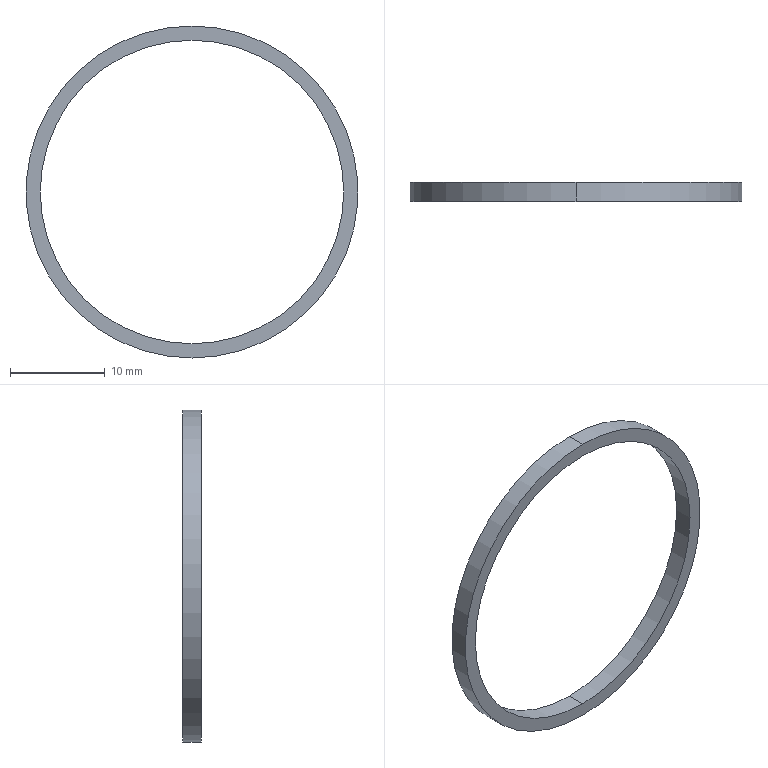Part | SolidWorks | features Extrusion 1 | 1 solid | 6 faces | box 35 x 2 x 35 mm | volume 315.73 mm3 | cylinder 4 | plane 2 | commonest cylinder face diameters 32 x2 35 x2
STEP:
#1=CARTESIAN_POINT('',(0.,1.,-16.));
#2=VERTEX_POINT('',#1);
#3=CARTESIAN_POINT('',(0.,1.,16.));
#4=VERTEX_POINT('',#3);
#5=CARTESIAN_POINT('',(0.,1.,0.));
#6=DIRECTION('',(0.,1.,0.));
#7=DIRECTION('',(0.,0.,1.));
#8=AXIS2_PLACEMENT_3D('',#5,#6,#7);
#9=CIRCLE('',#8,16.);
#10=EDGE_CURVE('',#2,#4,#9,.T.);
#11=ORIENTED_EDGE('',*,*,#10,.T.);
#12=CARTESIAN_POINT('',(0.,-1.,16.));
#13=VERTEX_POINT('',#12);
#14=CARTESIAN_POINT('',(0.,1.,16.));
#15=DIRECTION('',(0.,-1.,0.));
#16=VECTOR('',#15,1000.);
#17=LINE('',#14,#16);
#18=EDGE_CURVE('',#4,#13,#17,.T.);
#19=ORIENTED_EDGE('',*,*,#18,.T.);
#20=CARTESIAN_POINT('',(0.,-1.,-16.));
#21=VERTEX_POINT('',#20);
#22=CARTESIAN_POINT('',(0.,-1.,0.));
#23=DIRECTION('',(0.,1.,0.));
#24=DIRECTION('',(0.,0.,1.));
#25=AXIS2_PLACEMENT_3D('',#22,#23,#24);
#26=CIRCLE('',#25,16.);
#27=EDGE_CURVE('',#21,#13,#26,.T.);
#28=ORIENTED_EDGE('',*,*,#27,.F.);
#29=CARTESIAN_POINT('',(0.,1.,-16.));
#30=DIRECTION('',(0.,-1.,0.));
#31=VECTOR('',#30,1000.);
#32=LINE('',#29,#31);
#33=EDGE_CURVE('',#2,#21,#32,.T.);
#34=ORIENTED_EDGE('',*,*,#33,.F.);
#35=EDGE_LOOP('',(#11,#19,#28,#34));
#36=FACE_OUTER_BOUND('',#35,.T.);
#37=CARTESIAN_POINT('',(0.,1.,0.));
#38=DIRECTION('',(0.,-1.,0.));
#39=DIRECTION('',(0.,0.,-1.));
#40=AXIS2_PLACEMENT_3D('',#37,#38,#39);
#41=CYLINDRICAL_SURFACE('',#40,16.);
#42=ADVANCED_FACE('',(#36),#41,.F.);
#43=CARTESIAN_POINT('',(0.,1.,17.5));
#44=VERTEX_POINT('',#43);
#45=CARTESIAN_POINT('',(0.,1.,-17.5));
#46=VERTEX_POINT('',#45);
#47=CARTESIAN_POINT('',(0.,1.,0.));
#48=DIRECTION('',(0.,1.,0.));
#49=DIRECTION('',(0.,0.,1.));
#50=AXIS2_PLACEMENT_3D('',#47,#48,#49);
#51=CIRCLE('',#50,17.5);
#52=EDGE_CURVE('',#44,#46,#51,.T.);
#53=ORIENTED_EDGE('',*,*,#52,.F.);
#54=CARTESIAN_POINT('',(0.,-1.,17.5));
#55=VERTEX_POINT('',#54);
#56=CARTESIAN_POINT('',(0.,1.,17.5));
#57=DIRECTION('',(0.,-1.,0.));
#58=VECTOR('',#57,1000.);
#59=LINE('',#56,#58);
#60=EDGE_CURVE('',#44,#55,#59,.T.);
#61=ORIENTED_EDGE('',*,*,#60,.T.);
#62=CARTESIAN_POINT('',(0.,-1.,-17.5));
#63=VERTEX_POINT('',#62);
#64=CARTESIAN_POINT('',(0.,-1.,0.));
#65=DIRECTION('',(0.,1.,0.));
#66=DIRECTION('',(0.,0.,1.));
#67=AXIS2_PLACEMENT_3D('',#64,#65,#66);
#68=CIRCLE('',#67,17.5);
#69=EDGE_CURVE('',#55,#63,#68,.T.);
#70=ORIENTED_EDGE('',*,*,#69,.T.);
#71=CARTESIAN_POINT('',(0.,1.,-17.5));
#72=DIRECTION('',(0.,-1.,0.));
#73=VECTOR('',#72,1000.);
#74=LINE('',#71,#73);
#75=EDGE_CURVE('',#46,#63,#74,.T.);
#76=ORIENTED_EDGE('',*,*,#75,.F.);
#77=EDGE_LOOP('',(#53,#61,#70,#76));
#78=FACE_OUTER_BOUND('',#77,.T.);
#79=CARTESIAN_POINT('',(0.,1.,0.));
#80=DIRECTION('',(0.,-1.,0.));
#81=DIRECTION('',(0.,0.,-1.));
#82=AXIS2_PLACEMENT_3D('',#79,#80,#81);
#83=CYLINDRICAL_SURFACE('',#82,17.5);
#84=ADVANCED_FACE('',(#78),#83,.T.);
#85=CARTESIAN_POINT('',(0.,1.,0.));
#86=DIRECTION('',(0.,1.,0.));
#87=DIRECTION('',(0.,0.,1.));
#88=AXIS2_PLACEMENT_3D('',#85,#86,#87);
#89=CIRCLE('',#88,17.5);
#90=EDGE_CURVE('',#46,#44,#89,.T.);
#91=ORIENTED_EDGE('',*,*,#90,.T.);
#92=ORIENTED_EDGE('',*,*,#52,.T.);
#93=EDGE_LOOP('',(#91,#92));
#94=FACE_OUTER_BOUND('',#93,.T.);
#95=ORIENTED_EDGE('',*,*,#10,.F.);
#96=CARTESIAN_POINT('',(0.,1.,0.));
#97=DIRECTION('',(0.,1.,0.));
#98=DIRECTION('',(0.,0.,1.));
#99=AXIS2_PLACEMENT_3D('',#96,#97,#98);
#100=CIRCLE('',#99,16.);
#101=EDGE_CURVE('',#4,#2,#100,.T.);
#102=ORIENTED_EDGE('',*,*,#101,.F.);
#103=EDGE_LOOP('',(#95,#102));
#104=FACE_BOUND('',#103,.T.);
#105=CARTESIAN_POINT('',(0.,1.,0.));
#106=DIRECTION('',(0.,1.,0.));
#107=DIRECTION('',(0.,0.,1.));
#108=AXIS2_PLACEMENT_3D('',#105,#106,#107);
#109=PLANE('',#108);
#110=ADVANCED_FACE('',(#94,#104),#109,.T.);
#111=CARTESIAN_POINT('',(0.,-1.,0.));
#112=DIRECTION('',(0.,1.,0.));
#113=DIRECTION('',(0.,0.,1.));
#114=AXIS2_PLACEMENT_3D('',#111,#112,#113);
#115=CIRCLE('',#114,17.5);
#116=EDGE_CURVE('',#63,#55,#115,.T.);
#117=ORIENTED_EDGE('',*,*,#116,.F.);
#118=ORIENTED_EDGE('',*,*,#69,.F.);
#119=EDGE_LOOP('',(#117,#118));
#120=FACE_OUTER_BOUND('',#119,.T.);
#121=ORIENTED_EDGE('',*,*,#27,.T.);
#122=CARTESIAN_POINT('',(0.,-1.,0.));
#123=DIRECTION('',(0.,1.,0.));
#124=DIRECTION('',(0.,0.,1.));
#125=AXIS2_PLACEMENT_3D('',#122,#123,#124);
#126=CIRCLE('',#125,16.);
#127=EDGE_CURVE('',#13,#21,#126,.T.);
#128=ORIENTED_EDGE('',*,*,#127,.T.);
#129=EDGE_LOOP('',(#121,#128));
#130=FACE_BOUND('',#129,.T.);
#131=CARTESIAN_POINT('',(0.,-1.,0.));
#132=DIRECTION('',(0.,1.,0.));
#133=DIRECTION('',(0.,0.,1.));
#134=AXIS2_PLACEMENT_3D('',#131,#132,#133);
#135=PLANE('',#134);
#136=ADVANCED_FACE('',(#120,#130),#135,.F.);
#137=ORIENTED_EDGE('',*,*,#60,.F.);
#138=ORIENTED_EDGE('',*,*,#90,.F.);
#139=ORIENTED_EDGE('',*,*,#75,.T.);
#140=ORIENTED_EDGE('',*,*,#116,.T.);
#141=EDGE_LOOP('',(#137,#138,#139,#140));
#142=FACE_OUTER_BOUND('',#141,.T.);
#143=CARTESIAN_POINT('',(0.,1.,0.));
#144=DIRECTION('',(0.,-1.,0.));
#145=DIRECTION('',(0.,0.,-1.));
#146=AXIS2_PLACEMENT_3D('',#143,#144,#145);
#147=CYLINDRICAL_SURFACE('',#146,17.5);
#148=ADVANCED_FACE('',(#142),#147,.T.);
#149=ORIENTED_EDGE('',*,*,#18,.F.);
#150=ORIENTED_EDGE('',*,*,#101,.T.);
#151=ORIENTED_EDGE('',*,*,#33,.T.);
#152=ORIENTED_EDGE('',*,*,#127,.F.);
#153=EDGE_LOOP('',(#149,#150,#151,#152));
#154=FACE_OUTER_BOUND('',#153,.T.);
#155=CARTESIAN_POINT('',(0.,1.,0.));
#156=DIRECTION('',(0.,-1.,0.));
#157=DIRECTION('',(0.,0.,-1.));
#158=AXIS2_PLACEMENT_3D('',#155,#156,#157);
#159=CYLINDRICAL_SURFACE('',#158,16.);
#160=ADVANCED_FACE('',(#154),#159,.F.);
#161=CLOSED_SHELL('',(#42,#84,#110,#136,#148,#160));
#162=MANIFOLD_SOLID_BREP('',#161);
#163=CARTESIAN_POINT('',(0.,0.,0.));
#164=DIRECTION('',(0.,0.,1.));
#165=DIRECTION('',(1.,0.,0.));
#166=AXIS2_PLACEMENT_3D('',#163,#164,#165);
#167=(LENGTH_UNIT()NAMED_UNIT(*)SI_UNIT(.MILLI.,.METRE.));
#168=UNCERTAINTY_MEASURE_WITH_UNIT(LENGTH_MEASURE(0.00001),#167,'','');
#169=(NAMED_UNIT(*)PLANE_ANGLE_UNIT()SI_UNIT($,.RADIAN.));
#170=(NAMED_UNIT(*)SI_UNIT($,.STERADIAN.)SOLID_ANGLE_UNIT());
#171=(GEOMETRIC_REPRESENTATION_CONTEXT(3)GLOBAL_UNCERTAINTY_ASSIGNED_CONTEXT((#168))GLOBAL_UNIT_ASSIGNED_CONTEXT((#167,#169,#170))REPRESENTATION_CONTEXT('',''));
#172=ADVANCED_BREP_SHAPE_REPRESENTATION('',(#162,#166),#171);